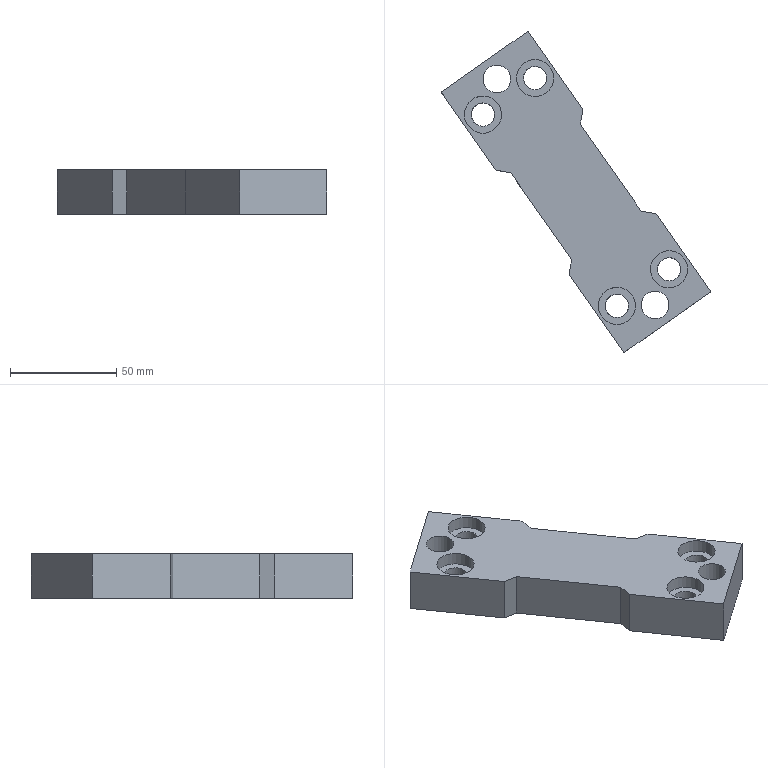Part | NX | features solid 2 | 1 solid | 28 faces | box 126.994 x 151.552 x 21 mm | volume 128901 mm3 | plane 18 | cylinder 10 | commonest cylinder face diameters 11 x4 17.5 x4 13 x2
STEP:
#1=CARTESIAN_POINT('',(-717.56,109.472,-44.));
#2=VERTEX_POINT('',#1);
#3=CARTESIAN_POINT('',(-722.579,116.64,-44.));
#4=DIRECTION('',(0.,0.,-1.));
#5=DIRECTION('',(0.5736,-0.8192,0.));
#6=AXIS2_PLACEMENT_3D('',#3,#4,#5);
#7=CIRCLE('',#6,8.75);
#8=EDGE_CURVE('',#2,#2,#7,.T.);
#9=ORIENTED_EDGE('',*,*,#8,.T.);
#10=EDGE_LOOP('',(#9));
#11=FACE_BOUND('',#10,.T.);
#12=CARTESIAN_POINT('',(-654.467,19.366,-44.));
#13=VERTEX_POINT('',#12);
#14=CARTESIAN_POINT('',(-659.485,26.533,-44.));
#15=DIRECTION('',(0.,0.,-1.));
#16=DIRECTION('',(0.5736,-0.8192,0.));
#17=AXIS2_PLACEMENT_3D('',#14,#15,#16);
#18=CIRCLE('',#17,8.75);
#19=EDGE_CURVE('',#13,#13,#18,.T.);
#20=ORIENTED_EDGE('',*,*,#19,.T.);
#21=EDGE_LOOP('',(#20));
#22=FACE_BOUND('',#21,.T.);
#23=CARTESIAN_POINT('',(-712.299,128.111,-44.));
#24=VERTEX_POINT('',#23);
#25=CARTESIAN_POINT('',(-716.027,133.435,-44.));
#26=DIRECTION('',(0.,0.,-1.));
#27=DIRECTION('',(0.5736,-0.8192,0.));
#28=AXIS2_PLACEMENT_3D('',#25,#26,#27);
#29=CIRCLE('',#28,6.5);
#30=EDGE_CURVE('',#24,#24,#29,.T.);
#31=ORIENTED_EDGE('',*,*,#30,.T.);
#32=EDGE_LOOP('',(#31));
#33=FACE_BOUND('',#32,.T.);
#34=CARTESIAN_POINT('',(-701.284,155.966,-44.));
#35=VERTEX_POINT('',#34);
#36=CARTESIAN_POINT('',(-742.242,127.287,-44.));
#37=VERTEX_POINT('',#36);
#38=CARTESIAN_POINT('',(-701.284,155.966,-44.));
#39=DIRECTION('',(-0.8192,-0.5736,0.));
#40=VECTOR('',#39,1000.);
#41=LINE('',#38,#40);
#42=EDGE_CURVE('',#35,#37,#41,.T.);
#43=ORIENTED_EDGE('',*,*,#42,.T.);
#44=CARTESIAN_POINT('',(-716.431,90.425,-44.));
#45=VERTEX_POINT('',#44);
#46=CARTESIAN_POINT('',(-742.242,127.287,-44.));
#47=DIRECTION('',(0.5736,-0.8192,0.));
#48=VECTOR('',#47,1000.);
#49=LINE('',#46,#48);
#50=EDGE_CURVE('',#37,#45,#49,.T.);
#51=ORIENTED_EDGE('',*,*,#50,.T.);
#52=CARTESIAN_POINT('',(-709.467,89.197,-44.));
#53=VERTEX_POINT('',#52);
#54=CARTESIAN_POINT('',(-716.431,90.425,-44.));
#55=DIRECTION('',(0.9848,-0.1736,0.));
#56=VECTOR('',#55,1000.);
#57=LINE('',#54,#56);
#58=EDGE_CURVE('',#45,#53,#57,.T.);
#59=ORIENTED_EDGE('',*,*,#58,.T.);
#60=CARTESIAN_POINT('',(-680.788,48.24,-44.));
#61=VERTEX_POINT('',#60);
#62=CARTESIAN_POINT('',(-709.467,89.197,-44.));
#63=DIRECTION('',(0.5736,-0.8192,0.));
#64=VECTOR('',#63,1000.);
#65=LINE('',#62,#64);
#66=EDGE_CURVE('',#53,#61,#65,.T.);
#67=ORIENTED_EDGE('',*,*,#66,.T.);
#68=CARTESIAN_POINT('',(-682.016,41.276,-44.));
#69=VERTEX_POINT('',#68);
#70=CARTESIAN_POINT('',(-680.788,48.24,-44.));
#71=DIRECTION('',(-0.1736,-0.9848,0.));
#72=VECTOR('',#71,1000.);
#73=LINE('',#70,#72);
#74=EDGE_CURVE('',#61,#69,#73,.T.);
#75=ORIENTED_EDGE('',*,*,#74,.T.);
#76=CARTESIAN_POINT('',(-656.205,4.414,-44.));
#77=VERTEX_POINT('',#76);
#78=CARTESIAN_POINT('',(-682.016,41.276,-44.));
#79=DIRECTION('',(0.5736,-0.8192,0.));
#80=VECTOR('',#79,1000.);
#81=LINE('',#78,#80);
#82=EDGE_CURVE('',#69,#77,#81,.T.);
#83=ORIENTED_EDGE('',*,*,#82,.T.);
#84=CARTESIAN_POINT('',(-615.248,33.093,-44.));
#85=VERTEX_POINT('',#84);
#86=CARTESIAN_POINT('',(-656.205,4.414,-44.));
#87=DIRECTION('',(0.8192,0.5736,0.));
#88=VECTOR('',#87,1000.);
#89=LINE('',#86,#88);
#90=EDGE_CURVE('',#77,#85,#89,.T.);
#91=ORIENTED_EDGE('',*,*,#90,.T.);
#92=CARTESIAN_POINT('',(-641.059,69.955,-44.));
#93=VERTEX_POINT('',#92);
#94=CARTESIAN_POINT('',(-641.059,69.955,-44.));
#95=DIRECTION('',(0.5736,-0.8192,0.));
#96=VECTOR('',#95,1000.);
#97=LINE('',#94,#96);
#98=EDGE_CURVE('',#93,#85,#97,.T.);
#99=ORIENTED_EDGE('',*,*,#98,.F.);
#100=CARTESIAN_POINT('',(-648.022,71.183,-44.));
#101=VERTEX_POINT('',#100);
#102=CARTESIAN_POINT('',(-648.022,71.183,-44.));
#103=DIRECTION('',(0.9848,-0.1736,0.));
#104=VECTOR('',#103,1000.);
#105=LINE('',#102,#104);
#106=EDGE_CURVE('',#101,#93,#105,.T.);
#107=ORIENTED_EDGE('',*,*,#106,.F.);
#108=CARTESIAN_POINT('',(-676.701,112.141,-44.));
#109=VERTEX_POINT('',#108);
#110=CARTESIAN_POINT('',(-676.701,112.141,-44.));
#111=DIRECTION('',(0.5736,-0.8192,0.));
#112=VECTOR('',#111,1000.);
#113=LINE('',#110,#112);
#114=EDGE_CURVE('',#109,#101,#113,.T.);
#115=ORIENTED_EDGE('',*,*,#114,.F.);
#116=CARTESIAN_POINT('',(-675.473,119.104,-44.));
#117=VERTEX_POINT('',#116);
#118=CARTESIAN_POINT('',(-676.701,112.141,-44.));
#119=DIRECTION('',(0.1736,0.9848,0.));
#120=VECTOR('',#119,1000.);
#121=LINE('',#118,#120);
#122=EDGE_CURVE('',#109,#117,#121,.T.);
#123=ORIENTED_EDGE('',*,*,#122,.T.);
#124=CARTESIAN_POINT('',(-701.284,155.966,-44.));
#125=DIRECTION('',(0.5736,-0.8192,0.));
#126=VECTOR('',#125,1000.);
#127=LINE('',#124,#126);
#128=EDGE_CURVE('',#35,#117,#127,.T.);
#129=ORIENTED_EDGE('',*,*,#128,.F.);
#130=EDGE_LOOP('',(#43,#51,#59,#67,#75,#83,#91,#99,#107,#115,#123,#129));
#131=FACE_BOUND('',#130,.T.);
#132=CARTESIAN_POINT('',(-637.734,21.621,-44.));
#133=VERTEX_POINT('',#132);
#134=CARTESIAN_POINT('',(-641.462,26.945,-44.));
#135=DIRECTION('',(0.,0.,-1.));
#136=DIRECTION('',(0.5736,-0.8192,0.));
#137=AXIS2_PLACEMENT_3D('',#134,#135,#136);
#138=CIRCLE('',#137,6.5);
#139=EDGE_CURVE('',#133,#133,#138,.T.);
#140=ORIENTED_EDGE('',*,*,#139,.T.);
#141=EDGE_LOOP('',(#140));
#142=FACE_BOUND('',#141,.T.);
#143=CARTESIAN_POINT('',(-629.892,36.573,-44.));
#144=VERTEX_POINT('',#143);
#145=CARTESIAN_POINT('',(-634.911,43.74,-44.));
#146=DIRECTION('',(0.,0.,-1.));
#147=DIRECTION('',(0.5736,-0.8192,0.));
#148=AXIS2_PLACEMENT_3D('',#145,#146,#147);
#149=CIRCLE('',#148,8.75);
#150=EDGE_CURVE('',#144,#144,#149,.T.);
#151=ORIENTED_EDGE('',*,*,#150,.T.);
#152=EDGE_LOOP('',(#151));
#153=FACE_BOUND('',#152,.T.);
#154=CARTESIAN_POINT('',(-692.985,126.68,-44.));
#155=VERTEX_POINT('',#154);
#156=CARTESIAN_POINT('',(-698.004,133.847,-44.));
#157=DIRECTION('',(0.,0.,-1.));
#158=DIRECTION('',(0.5736,-0.8192,0.));
#159=AXIS2_PLACEMENT_3D('',#156,#157,#158);
#160=CIRCLE('',#159,8.75);
#161=EDGE_CURVE('',#155,#155,#160,.T.);
#162=ORIENTED_EDGE('',*,*,#161,.T.);
#163=EDGE_LOOP('',(#162));
#164=FACE_BOUND('',#163,.T.);
#165=CARTESIAN_POINT('',(-742.242,127.287,-44.));
#166=DIRECTION('',(0.,0.,-1.));
#167=DIRECTION('',(-0.8192,-0.5736,0.));
#168=AXIS2_PLACEMENT_3D('',#165,#166,#167);
#169=PLANE('',#168);
#170=ADVANCED_FACE('',(#11,#22,#33,#131,#142,#153,#164),#169,.F.);
#171=CARTESIAN_POINT('',(-694.85,129.342,-65.));
#172=VERTEX_POINT('',#171);
#173=CARTESIAN_POINT('',(-698.004,133.847,-65.));
#174=DIRECTION('',(0.,0.,-1.));
#175=DIRECTION('',(0.5736,-0.8192,0.));
#176=AXIS2_PLACEMENT_3D('',#173,#174,#175);
#177=CIRCLE('',#176,5.5);
#178=EDGE_CURVE('',#172,#172,#177,.T.);
#179=ORIENTED_EDGE('',*,*,#178,.T.);
#180=EDGE_LOOP('',(#179));
#181=FACE_BOUND('',#180,.T.);
#182=CARTESIAN_POINT('',(-693.499,137.002,-50.));
#183=VERTEX_POINT('',#182);
#184=CARTESIAN_POINT('',(-698.004,133.847,-50.));
#185=DIRECTION('',(0.,0.,-1.));
#186=DIRECTION('',(0.8192,0.5736,0.));
#187=AXIS2_PLACEMENT_3D('',#184,#185,#186);
#188=CIRCLE('',#187,5.5);
#189=EDGE_CURVE('',#183,#183,#188,.T.);
#190=ORIENTED_EDGE('',*,*,#189,.F.);
#191=EDGE_LOOP('',(#190));
#192=FACE_BOUND('',#191,.T.);
#193=CARTESIAN_POINT('',(-698.004,133.847,-44.));
#194=DIRECTION('',(0.,0.,-1.));
#195=DIRECTION('',(-0.8192,-0.5736,0.));
#196=AXIS2_PLACEMENT_3D('',#193,#194,#195);
#197=CYLINDRICAL_SURFACE('',#196,5.5);
#198=ADVANCED_FACE('',(#181,#192),#197,.F.);
#199=CARTESIAN_POINT('',(-719.424,112.135,-65.));
#200=VERTEX_POINT('',#199);
#201=CARTESIAN_POINT('',(-722.579,116.64,-65.));
#202=DIRECTION('',(0.,0.,-1.));
#203=DIRECTION('',(0.5736,-0.8192,0.));
#204=AXIS2_PLACEMENT_3D('',#201,#202,#203);
#205=CIRCLE('',#204,5.5);
#206=EDGE_CURVE('',#200,#200,#205,.T.);
#207=ORIENTED_EDGE('',*,*,#206,.T.);
#208=EDGE_LOOP('',(#207));
#209=FACE_BOUND('',#208,.T.);
#210=CARTESIAN_POINT('',(-718.073,119.795,-50.));
#211=VERTEX_POINT('',#210);
#212=CARTESIAN_POINT('',(-722.579,116.64,-50.));
#213=DIRECTION('',(0.,0.,-1.));
#214=DIRECTION('',(0.8192,0.5736,0.));
#215=AXIS2_PLACEMENT_3D('',#212,#213,#214);
#216=CIRCLE('',#215,5.5);
#217=EDGE_CURVE('',#211,#211,#216,.T.);
#218=ORIENTED_EDGE('',*,*,#217,.F.);
#219=EDGE_LOOP('',(#218));
#220=FACE_BOUND('',#219,.T.);
#221=CARTESIAN_POINT('',(-722.579,116.64,-44.));
#222=DIRECTION('',(0.,0.,-1.));
#223=DIRECTION('',(-0.8192,-0.5736,0.));
#224=AXIS2_PLACEMENT_3D('',#221,#222,#223);
#225=CYLINDRICAL_SURFACE('',#224,5.5);
#226=ADVANCED_FACE('',(#209,#220),#225,.F.);
#227=CARTESIAN_POINT('',(-631.756,39.235,-65.));
#228=VERTEX_POINT('',#227);
#229=CARTESIAN_POINT('',(-634.911,43.74,-65.));
#230=DIRECTION('',(0.,0.,-1.));
#231=DIRECTION('',(0.5736,-0.8192,0.));
#232=AXIS2_PLACEMENT_3D('',#229,#230,#231);
#233=CIRCLE('',#232,5.5);
#234=EDGE_CURVE('',#228,#228,#233,.T.);
#235=ORIENTED_EDGE('',*,*,#234,.T.);
#236=EDGE_LOOP('',(#235));
#237=FACE_BOUND('',#236,.T.);
#238=CARTESIAN_POINT('',(-630.406,46.895,-50.));
#239=VERTEX_POINT('',#238);
#240=CARTESIAN_POINT('',(-634.911,43.74,-50.));
#241=DIRECTION('',(0.,0.,-1.));
#242=DIRECTION('',(0.8192,0.5736,0.));
#243=AXIS2_PLACEMENT_3D('',#240,#241,#242);
#244=CIRCLE('',#243,5.5);
#245=EDGE_CURVE('',#239,#239,#244,.T.);
#246=ORIENTED_EDGE('',*,*,#245,.F.);
#247=EDGE_LOOP('',(#246));
#248=FACE_BOUND('',#247,.T.);
#249=CARTESIAN_POINT('',(-634.911,43.74,-44.));
#250=DIRECTION('',(0.,0.,-1.));
#251=DIRECTION('',(-0.8192,-0.5736,0.));
#252=AXIS2_PLACEMENT_3D('',#249,#250,#251);
#253=CYLINDRICAL_SURFACE('',#252,5.5);
#254=ADVANCED_FACE('',(#237,#248),#253,.F.);
#255=CARTESIAN_POINT('',(-656.331,22.028,-65.));
#256=VERTEX_POINT('',#255);
#257=CARTESIAN_POINT('',(-659.485,26.533,-65.));
#258=DIRECTION('',(0.,0.,-1.));
#259=DIRECTION('',(0.5736,-0.8192,0.));
#260=AXIS2_PLACEMENT_3D('',#257,#258,#259);
#261=CIRCLE('',#260,5.5);
#262=EDGE_CURVE('',#256,#256,#261,.T.);
#263=ORIENTED_EDGE('',*,*,#262,.T.);
#264=EDGE_LOOP('',(#263));
#265=FACE_BOUND('',#264,.T.);
#266=CARTESIAN_POINT('',(-654.98,29.688,-50.));
#267=VERTEX_POINT('',#266);
#268=CARTESIAN_POINT('',(-659.485,26.533,-50.));
#269=DIRECTION('',(0.,0.,-1.));
#270=DIRECTION('',(0.8192,0.5736,0.));
#271=AXIS2_PLACEMENT_3D('',#268,#269,#270);
#272=CIRCLE('',#271,5.5);
#273=EDGE_CURVE('',#267,#267,#272,.T.);
#274=ORIENTED_EDGE('',*,*,#273,.F.);
#275=EDGE_LOOP('',(#274));
#276=FACE_BOUND('',#275,.T.);
#277=CARTESIAN_POINT('',(-659.485,26.533,-44.));
#278=DIRECTION('',(0.,0.,-1.));
#279=DIRECTION('',(-0.8192,-0.5736,0.));
#280=AXIS2_PLACEMENT_3D('',#277,#278,#279);
#281=CYLINDRICAL_SURFACE('',#280,5.5);
#282=ADVANCED_FACE('',(#265,#276),#281,.F.);
#283=CARTESIAN_POINT('',(-712.299,128.111,-65.));
#284=VERTEX_POINT('',#283);
#285=CARTESIAN_POINT('',(-716.027,133.435,-65.));
#286=DIRECTION('',(0.,0.,-1.));
#287=DIRECTION('',(0.5736,-0.8192,0.));
#288=AXIS2_PLACEMENT_3D('',#285,#286,#287);
#289=CIRCLE('',#288,6.5);
#290=EDGE_CURVE('',#284,#284,#289,.T.);
#291=ORIENTED_EDGE('',*,*,#290,.F.);
#292=EDGE_LOOP('',(#291));
#293=FACE_BOUND('',#292,.T.);
#294=ORIENTED_EDGE('',*,*,#234,.F.);
#295=EDGE_LOOP('',(#294));
#296=FACE_BOUND('',#295,.T.);
#297=ORIENTED_EDGE('',*,*,#262,.F.);
#298=EDGE_LOOP('',(#297));
#299=FACE_BOUND('',#298,.T.);
#300=CARTESIAN_POINT('',(-701.284,155.966,-65.));
#301=VERTEX_POINT('',#300);
#302=CARTESIAN_POINT('',(-742.242,127.287,-65.));
#303=VERTEX_POINT('',#302);
#304=CARTESIAN_POINT('',(-701.284,155.966,-65.));
#305=DIRECTION('',(-0.8192,-0.5736,0.));
#306=VECTOR('',#305,1000.);
#307=LINE('',#304,#306);
#308=EDGE_CURVE('',#301,#303,#307,.T.);
#309=ORIENTED_EDGE('',*,*,#308,.F.);
#310=CARTESIAN_POINT('',(-675.473,119.104,-65.));
#311=VERTEX_POINT('',#310);
#312=CARTESIAN_POINT('',(-701.284,155.966,-65.));
#313=DIRECTION('',(0.5736,-0.8192,0.));
#314=VECTOR('',#313,1000.);
#315=LINE('',#312,#314);
#316=EDGE_CURVE('',#301,#311,#315,.T.);
#317=ORIENTED_EDGE('',*,*,#316,.T.);
#318=CARTESIAN_POINT('',(-676.701,112.141,-65.));
#319=VERTEX_POINT('',#318);
#320=CARTESIAN_POINT('',(-676.701,112.141,-65.));
#321=DIRECTION('',(0.1736,0.9848,0.));
#322=VECTOR('',#321,1000.);
#323=LINE('',#320,#322);
#324=EDGE_CURVE('',#319,#311,#323,.T.);
#325=ORIENTED_EDGE('',*,*,#324,.F.);
#326=CARTESIAN_POINT('',(-648.022,71.183,-65.));
#327=VERTEX_POINT('',#326);
#328=CARTESIAN_POINT('',(-676.701,112.141,-65.));
#329=DIRECTION('',(0.5736,-0.8192,0.));
#330=VECTOR('',#329,1000.);
#331=LINE('',#328,#330);
#332=EDGE_CURVE('',#319,#327,#331,.T.);
#333=ORIENTED_EDGE('',*,*,#332,.T.);
#334=CARTESIAN_POINT('',(-641.059,69.955,-65.));
#335=VERTEX_POINT('',#334);
#336=CARTESIAN_POINT('',(-648.022,71.183,-65.));
#337=DIRECTION('',(0.9848,-0.1736,0.));
#338=VECTOR('',#337,1000.);
#339=LINE('',#336,#338);
#340=EDGE_CURVE('',#327,#335,#339,.T.);
#341=ORIENTED_EDGE('',*,*,#340,.T.);
#342=CARTESIAN_POINT('',(-615.248,33.093,-65.));
#343=VERTEX_POINT('',#342);
#344=CARTESIAN_POINT('',(-641.059,69.955,-65.));
#345=DIRECTION('',(0.5736,-0.8192,0.));
#346=VECTOR('',#345,1000.);
#347=LINE('',#344,#346);
#348=EDGE_CURVE('',#335,#343,#347,.T.);
#349=ORIENTED_EDGE('',*,*,#348,.T.);
#350=CARTESIAN_POINT('',(-656.205,4.414,-65.));
#351=VERTEX_POINT('',#350);
#352=CARTESIAN_POINT('',(-656.205,4.414,-65.));
#353=DIRECTION('',(0.8192,0.5736,0.));
#354=VECTOR('',#353,1000.);
#355=LINE('',#352,#354);
#356=EDGE_CURVE('',#351,#343,#355,.T.);
#357=ORIENTED_EDGE('',*,*,#356,.F.);
#358=CARTESIAN_POINT('',(-682.016,41.276,-65.));
#359=VERTEX_POINT('',#358);
#360=CARTESIAN_POINT('',(-682.016,41.276,-65.));
#361=DIRECTION('',(0.5736,-0.8192,0.));
#362=VECTOR('',#361,1000.);
#363=LINE('',#360,#362);
#364=EDGE_CURVE('',#359,#351,#363,.T.);
#365=ORIENTED_EDGE('',*,*,#364,.F.);
#366=CARTESIAN_POINT('',(-680.788,48.24,-65.));
#367=VERTEX_POINT('',#366);
#368=CARTESIAN_POINT('',(-680.788,48.24,-65.));
#369=DIRECTION('',(-0.1736,-0.9848,0.));
#370=VECTOR('',#369,1000.);
#371=LINE('',#368,#370);
#372=EDGE_CURVE('',#367,#359,#371,.T.);
#373=ORIENTED_EDGE('',*,*,#372,.F.);
#374=CARTESIAN_POINT('',(-709.467,89.197,-65.));
#375=VERTEX_POINT('',#374);
#376=CARTESIAN_POINT('',(-709.467,89.197,-65.));
#377=DIRECTION('',(0.5736,-0.8192,0.));
#378=VECTOR('',#377,1000.);
#379=LINE('',#376,#378);
#380=EDGE_CURVE('',#375,#367,#379,.T.);
#381=ORIENTED_EDGE('',*,*,#380,.F.);
#382=CARTESIAN_POINT('',(-716.431,90.425,-65.));
#383=VERTEX_POINT('',#382);
#384=CARTESIAN_POINT('',(-716.431,90.425,-65.));
#385=DIRECTION('',(0.9848,-0.1736,0.));
#386=VECTOR('',#385,1000.);
#387=LINE('',#384,#386);
#388=EDGE_CURVE('',#383,#375,#387,.T.);
#389=ORIENTED_EDGE('',*,*,#388,.F.);
#390=CARTESIAN_POINT('',(-742.242,127.287,-65.));
#391=DIRECTION('',(0.5736,-0.8192,0.));
#392=VECTOR('',#391,1000.);
#393=LINE('',#390,#392);
#394=EDGE_CURVE('',#303,#383,#393,.T.);
#395=ORIENTED_EDGE('',*,*,#394,.F.);
#396=EDGE_LOOP('',(#309,#317,#325,#333,#341,#349,#357,#365,#373,#381,#389,#395));
#397=FACE_BOUND('',#396,.T.);
#398=CARTESIAN_POINT('',(-637.734,21.621,-65.));
#399=VERTEX_POINT('',#398);
#400=CARTESIAN_POINT('',(-641.462,26.945,-65.));
#401=DIRECTION('',(0.,0.,-1.));
#402=DIRECTION('',(0.5736,-0.8192,0.));
#403=AXIS2_PLACEMENT_3D('',#400,#401,#402);
#404=CIRCLE('',#403,6.5);
#405=EDGE_CURVE('',#399,#399,#404,.T.);
#406=ORIENTED_EDGE('',*,*,#405,.F.);
#407=EDGE_LOOP('',(#406));
#408=FACE_BOUND('',#407,.T.);
#409=ORIENTED_EDGE('',*,*,#206,.F.);
#410=EDGE_LOOP('',(#409));
#411=FACE_BOUND('',#410,.T.);
#412=ORIENTED_EDGE('',*,*,#178,.F.);
#413=EDGE_LOOP('',(#412));
#414=FACE_BOUND('',#413,.T.);
#415=CARTESIAN_POINT('',(-742.242,127.287,-65.));
#416=DIRECTION('',(0.,0.,-1.));
#417=DIRECTION('',(-0.8192,-0.5736,0.));
#418=AXIS2_PLACEMENT_3D('',#415,#416,#417);
#419=PLANE('',#418);
#420=ADVANCED_FACE('',(#293,#296,#299,#397,#408,#411,#414),#419,.T.);
#421=ORIENTED_EDGE('',*,*,#308,.T.);
#422=CARTESIAN_POINT('',(-742.242,127.287,-44.));
#423=DIRECTION('',(0.,0.,-1.));
#424=VECTOR('',#423,1000.);
#425=LINE('',#422,#424);
#426=EDGE_CURVE('',#37,#303,#425,.T.);
#427=ORIENTED_EDGE('',*,*,#426,.F.);
#428=ORIENTED_EDGE('',*,*,#42,.F.);
#429=CARTESIAN_POINT('',(-701.284,155.966,-44.));
#430=DIRECTION('',(0.,0.,-1.));
#431=VECTOR('',#430,1000.);
#432=LINE('',#429,#431);
#433=EDGE_CURVE('',#35,#301,#432,.T.);
#434=ORIENTED_EDGE('',*,*,#433,.T.);
#435=EDGE_LOOP('',(#421,#427,#428,#434));
#436=FACE_BOUND('',#435,.T.);
#437=CARTESIAN_POINT('',(-701.284,155.966,-44.));
#438=DIRECTION('',(-0.5736,0.8192,0.));
#439=DIRECTION('',(0.8192,0.5736,0.));
#440=AXIS2_PLACEMENT_3D('',#437,#438,#439);
#441=PLANE('',#440);
#442=ADVANCED_FACE('',(#436),#441,.T.);
#443=ORIENTED_EDGE('',*,*,#394,.T.);
#444=CARTESIAN_POINT('',(-716.431,90.425,-44.));
#445=DIRECTION('',(0.,0.,-1.));
#446=VECTOR('',#445,1000.);
#447=LINE('',#444,#446);
#448=EDGE_CURVE('',#45,#383,#447,.T.);
#449=ORIENTED_EDGE('',*,*,#448,.F.);
#450=ORIENTED_EDGE('',*,*,#50,.F.);
#451=ORIENTED_EDGE('',*,*,#426,.T.);
#452=EDGE_LOOP('',(#443,#449,#450,#451));
#453=FACE_BOUND('',#452,.T.);
#454=CARTESIAN_POINT('',(-742.242,127.287,-44.));
#455=DIRECTION('',(-0.8192,-0.5736,0.));
#456=DIRECTION('',(-0.5736,0.8192,0.));
#457=AXIS2_PLACEMENT_3D('',#454,#455,#456);
#458=PLANE('',#457);
#459=ADVANCED_FACE('',(#453),#458,.T.);
#460=ORIENTED_EDGE('',*,*,#388,.T.);
#461=CARTESIAN_POINT('',(-709.467,89.197,-44.));
#462=DIRECTION('',(0.,0.,-1.));
#463=VECTOR('',#462,1000.);
#464=LINE('',#461,#463);
#465=EDGE_CURVE('',#53,#375,#464,.T.);
#466=ORIENTED_EDGE('',*,*,#465,.F.);
#467=ORIENTED_EDGE('',*,*,#58,.F.);
#468=ORIENTED_EDGE('',*,*,#448,.T.);
#469=EDGE_LOOP('',(#460,#466,#467,#468));
#470=FACE_BOUND('',#469,.T.);
#471=CARTESIAN_POINT('',(-716.431,90.425,-44.));
#472=DIRECTION('',(-0.1736,-0.9848,0.));
#473=DIRECTION('',(-0.9848,0.1736,0.));
#474=AXIS2_PLACEMENT_3D('',#471,#472,#473);
#475=PLANE('',#474);
#476=ADVANCED_FACE('',(#470),#475,.T.);
#477=ORIENTED_EDGE('',*,*,#380,.T.);
#478=CARTESIAN_POINT('',(-680.788,48.24,-44.));
#479=DIRECTION('',(0.,0.,-1.));
#480=VECTOR('',#479,1000.);
#481=LINE('',#478,#480);
#482=EDGE_CURVE('',#61,#367,#481,.T.);
#483=ORIENTED_EDGE('',*,*,#482,.F.);
#484=ORIENTED_EDGE('',*,*,#66,.F.);
#485=ORIENTED_EDGE('',*,*,#465,.T.);
#486=EDGE_LOOP('',(#477,#483,#484,#485));
#487=FACE_BOUND('',#486,.T.);
#488=CARTESIAN_POINT('',(-709.467,89.197,-44.));
#489=DIRECTION('',(-0.8192,-0.5736,0.));
#490=DIRECTION('',(-0.5736,0.8192,0.));
#491=AXIS2_PLACEMENT_3D('',#488,#489,#490);
#492=PLANE('',#491);
#493=ADVANCED_FACE('',(#487),#492,.T.);
#494=ORIENTED_EDGE('',*,*,#372,.T.);
#495=CARTESIAN_POINT('',(-682.016,41.276,-44.));
#496=DIRECTION('',(0.,0.,-1.));
#497=VECTOR('',#496,1000.);
#498=LINE('',#495,#497);
#499=EDGE_CURVE('',#69,#359,#498,.T.);
#500=ORIENTED_EDGE('',*,*,#499,.F.);
#501=ORIENTED_EDGE('',*,*,#74,.F.);
#502=ORIENTED_EDGE('',*,*,#482,.T.);
#503=EDGE_LOOP('',(#494,#500,#501,#502));
#504=FACE_BOUND('',#503,.T.);
#505=CARTESIAN_POINT('',(-680.788,48.24,-44.));
#506=DIRECTION('',(-0.9848,0.1736,0.));
#507=DIRECTION('',(0.1736,0.9848,0.));
#508=AXIS2_PLACEMENT_3D('',#505,#506,#507);
#509=PLANE('',#508);
#510=ADVANCED_FACE('',(#504),#509,.T.);
#511=ORIENTED_EDGE('',*,*,#364,.T.);
#512=CARTESIAN_POINT('',(-656.205,4.414,-44.));
#513=DIRECTION('',(0.,0.,-1.));
#514=VECTOR('',#513,1000.);
#515=LINE('',#512,#514);
#516=EDGE_CURVE('',#77,#351,#515,.T.);
#517=ORIENTED_EDGE('',*,*,#516,.F.);
#518=ORIENTED_EDGE('',*,*,#82,.F.);
#519=ORIENTED_EDGE('',*,*,#499,.T.);
#520=EDGE_LOOP('',(#511,#517,#518,#519));
#521=FACE_BOUND('',#520,.T.);
#522=CARTESIAN_POINT('',(-682.016,41.276,-44.));
#523=DIRECTION('',(-0.8192,-0.5736,0.));
#524=DIRECTION('',(-0.5736,0.8192,0.));
#525=AXIS2_PLACEMENT_3D('',#522,#523,#524);
#526=PLANE('',#525);
#527=ADVANCED_FACE('',(#521),#526,.T.);
#528=ORIENTED_EDGE('',*,*,#356,.T.);
#529=CARTESIAN_POINT('',(-615.248,33.093,-44.));
#530=DIRECTION('',(0.,0.,-1.));
#531=VECTOR('',#530,1000.);
#532=LINE('',#529,#531);
#533=EDGE_CURVE('',#85,#343,#532,.T.);
#534=ORIENTED_EDGE('',*,*,#533,.F.);
#535=ORIENTED_EDGE('',*,*,#90,.F.);
#536=ORIENTED_EDGE('',*,*,#516,.T.);
#537=EDGE_LOOP('',(#528,#534,#535,#536));
#538=FACE_BOUND('',#537,.T.);
#539=CARTESIAN_POINT('',(-656.205,4.414,-44.));
#540=DIRECTION('',(0.5736,-0.8192,0.));
#541=DIRECTION('',(-0.8192,-0.5736,0.));
#542=AXIS2_PLACEMENT_3D('',#539,#540,#541);
#543=PLANE('',#542);
#544=ADVANCED_FACE('',(#538),#543,.T.);
#545=ORIENTED_EDGE('',*,*,#348,.F.);
#546=CARTESIAN_POINT('',(-641.059,69.955,-44.));
#547=DIRECTION('',(0.,0.,-1.));
#548=VECTOR('',#547,1000.);
#549=LINE('',#546,#548);
#550=EDGE_CURVE('',#93,#335,#549,.T.);
#551=ORIENTED_EDGE('',*,*,#550,.F.);
#552=ORIENTED_EDGE('',*,*,#98,.T.);
#553=ORIENTED_EDGE('',*,*,#533,.T.);
#554=EDGE_LOOP('',(#545,#551,#552,#553));
#555=FACE_BOUND('',#554,.T.);
#556=CARTESIAN_POINT('',(-641.059,69.955,-44.));
#557=DIRECTION('',(-0.8192,-0.5736,0.));
#558=DIRECTION('',(-0.5736,0.8192,0.));
#559=AXIS2_PLACEMENT_3D('',#556,#557,#558);
#560=PLANE('',#559);
#561=ADVANCED_FACE('',(#555),#560,.F.);
#562=ORIENTED_EDGE('',*,*,#340,.F.);
#563=CARTESIAN_POINT('',(-648.022,71.183,-44.));
#564=DIRECTION('',(0.,0.,-1.));
#565=VECTOR('',#564,1000.);
#566=LINE('',#563,#565);
#567=EDGE_CURVE('',#101,#327,#566,.T.);
#568=ORIENTED_EDGE('',*,*,#567,.F.);
#569=ORIENTED_EDGE('',*,*,#106,.T.);
#570=ORIENTED_EDGE('',*,*,#550,.T.);
#571=EDGE_LOOP('',(#562,#568,#569,#570));
#572=FACE_BOUND('',#571,.T.);
#573=CARTESIAN_POINT('',(-648.022,71.183,-44.));
#574=DIRECTION('',(-0.1736,-0.9848,0.));
#575=DIRECTION('',(-0.9848,0.1736,0.));
#576=AXIS2_PLACEMENT_3D('',#573,#574,#575);
#577=PLANE('',#576);
#578=ADVANCED_FACE('',(#572),#577,.F.);
#579=ORIENTED_EDGE('',*,*,#332,.F.);
#580=CARTESIAN_POINT('',(-676.701,112.141,-44.));
#581=DIRECTION('',(0.,0.,-1.));
#582=VECTOR('',#581,1000.);
#583=LINE('',#580,#582);
#584=EDGE_CURVE('',#109,#319,#583,.T.);
#585=ORIENTED_EDGE('',*,*,#584,.F.);
#586=ORIENTED_EDGE('',*,*,#114,.T.);
#587=ORIENTED_EDGE('',*,*,#567,.T.);
#588=EDGE_LOOP('',(#579,#585,#586,#587));
#589=FACE_BOUND('',#588,.T.);
#590=CARTESIAN_POINT('',(-676.701,112.141,-44.));
#591=DIRECTION('',(-0.8192,-0.5736,0.));
#592=DIRECTION('',(-0.5736,0.8192,0.));
#593=AXIS2_PLACEMENT_3D('',#590,#591,#592);
#594=PLANE('',#593);
#595=ADVANCED_FACE('',(#589),#594,.F.);
#596=ORIENTED_EDGE('',*,*,#324,.T.);
#597=CARTESIAN_POINT('',(-675.473,119.104,-44.));
#598=DIRECTION('',(0.,0.,-1.));
#599=VECTOR('',#598,1000.);
#600=LINE('',#597,#599);
#601=EDGE_CURVE('',#117,#311,#600,.T.);
#602=ORIENTED_EDGE('',*,*,#601,.F.);
#603=ORIENTED_EDGE('',*,*,#122,.F.);
#604=ORIENTED_EDGE('',*,*,#584,.T.);
#605=EDGE_LOOP('',(#596,#602,#603,#604));
#606=FACE_BOUND('',#605,.T.);
#607=CARTESIAN_POINT('',(-676.701,112.141,-44.));
#608=DIRECTION('',(0.9848,-0.1736,0.));
#609=DIRECTION('',(-0.1736,-0.9848,0.));
#610=AXIS2_PLACEMENT_3D('',#607,#608,#609);
#611=PLANE('',#610);
#612=ADVANCED_FACE('',(#606),#611,.T.);
#613=ORIENTED_EDGE('',*,*,#316,.F.);
#614=ORIENTED_EDGE('',*,*,#433,.F.);
#615=ORIENTED_EDGE('',*,*,#128,.T.);
#616=ORIENTED_EDGE('',*,*,#601,.T.);
#617=EDGE_LOOP('',(#613,#614,#615,#616));
#618=FACE_BOUND('',#617,.T.);
#619=CARTESIAN_POINT('',(-701.284,155.966,-44.));
#620=DIRECTION('',(-0.8192,-0.5736,0.));
#621=DIRECTION('',(-0.5736,0.8192,0.));
#622=AXIS2_PLACEMENT_3D('',#619,#620,#621);
#623=PLANE('',#622);
#624=ADVANCED_FACE('',(#618),#623,.F.);
#625=ORIENTED_EDGE('',*,*,#139,.F.);
#626=EDGE_LOOP('',(#625));
#627=FACE_BOUND('',#626,.T.);
#628=ORIENTED_EDGE('',*,*,#405,.T.);
#629=EDGE_LOOP('',(#628));
#630=FACE_BOUND('',#629,.T.);
#631=CARTESIAN_POINT('',(-641.462,26.945,-44.));
#632=DIRECTION('',(0.,0.,-1.));
#633=DIRECTION('',(-0.8192,-0.5736,0.));
#634=AXIS2_PLACEMENT_3D('',#631,#632,#633);
#635=CYLINDRICAL_SURFACE('',#634,6.5);
#636=ADVANCED_FACE('',(#627,#630),#635,.F.);
#637=ORIENTED_EDGE('',*,*,#30,.F.);
#638=EDGE_LOOP('',(#637));
#639=FACE_BOUND('',#638,.T.);
#640=ORIENTED_EDGE('',*,*,#290,.T.);
#641=EDGE_LOOP('',(#640));
#642=FACE_BOUND('',#641,.T.);
#643=CARTESIAN_POINT('',(-716.027,133.435,-44.));
#644=DIRECTION('',(0.,0.,-1.));
#645=DIRECTION('',(-0.8192,-0.5736,0.));
#646=AXIS2_PLACEMENT_3D('',#643,#644,#645);
#647=CYLINDRICAL_SURFACE('',#646,6.5);
#648=ADVANCED_FACE('',(#639,#642),#647,.F.);
#649=ORIENTED_EDGE('',*,*,#19,.F.);
#650=EDGE_LOOP('',(#649));
#651=FACE_BOUND('',#650,.T.);
#652=CARTESIAN_POINT('',(-654.467,19.366,-50.));
#653=VERTEX_POINT('',#652);
#654=CARTESIAN_POINT('',(-659.485,26.533,-50.));
#655=DIRECTION('',(0.,0.,-1.));
#656=DIRECTION('',(0.5736,-0.8192,0.));
#657=AXIS2_PLACEMENT_3D('',#654,#655,#656);
#658=CIRCLE('',#657,8.75);
#659=EDGE_CURVE('',#653,#653,#658,.T.);
#660=ORIENTED_EDGE('',*,*,#659,.T.);
#661=EDGE_LOOP('',(#660));
#662=FACE_BOUND('',#661,.T.);
#663=CARTESIAN_POINT('',(-659.485,26.533,-44.));
#664=DIRECTION('',(0.,0.,-1.));
#665=DIRECTION('',(-0.8192,-0.5736,0.));
#666=AXIS2_PLACEMENT_3D('',#663,#664,#665);
#667=CYLINDRICAL_SURFACE('',#666,8.75);
#668=ADVANCED_FACE('',(#651,#662),#667,.F.);
#669=ORIENTED_EDGE('',*,*,#273,.T.);
#670=EDGE_LOOP('',(#669));
#671=FACE_BOUND('',#670,.T.);
#672=ORIENTED_EDGE('',*,*,#659,.F.);
#673=EDGE_LOOP('',(#672));
#674=FACE_BOUND('',#673,.T.);
#675=CARTESIAN_POINT('',(-659.485,26.533,-50.));
#676=DIRECTION('',(0.,0.,1.));
#677=DIRECTION('',(0.8192,0.5736,0.));
#678=AXIS2_PLACEMENT_3D('',#675,#676,#677);
#679=PLANE('',#678);
#680=ADVANCED_FACE('',(#671,#674),#679,.T.);
#681=ORIENTED_EDGE('',*,*,#150,.F.);
#682=EDGE_LOOP('',(#681));
#683=FACE_BOUND('',#682,.T.);
#684=CARTESIAN_POINT('',(-629.892,36.573,-50.));
#685=VERTEX_POINT('',#684);
#686=CARTESIAN_POINT('',(-634.911,43.74,-50.));
#687=DIRECTION('',(0.,0.,-1.));
#688=DIRECTION('',(0.5736,-0.8192,0.));
#689=AXIS2_PLACEMENT_3D('',#686,#687,#688);
#690=CIRCLE('',#689,8.75);
#691=EDGE_CURVE('',#685,#685,#690,.T.);
#692=ORIENTED_EDGE('',*,*,#691,.T.);
#693=EDGE_LOOP('',(#692));
#694=FACE_BOUND('',#693,.T.);
#695=CARTESIAN_POINT('',(-634.911,43.74,-44.));
#696=DIRECTION('',(0.,0.,-1.));
#697=DIRECTION('',(-0.8192,-0.5736,0.));
#698=AXIS2_PLACEMENT_3D('',#695,#696,#697);
#699=CYLINDRICAL_SURFACE('',#698,8.75);
#700=ADVANCED_FACE('',(#683,#694),#699,.F.);
#701=ORIENTED_EDGE('',*,*,#245,.T.);
#702=EDGE_LOOP('',(#701));
#703=FACE_BOUND('',#702,.T.);
#704=ORIENTED_EDGE('',*,*,#691,.F.);
#705=EDGE_LOOP('',(#704));
#706=FACE_BOUND('',#705,.T.);
#707=CARTESIAN_POINT('',(-634.911,43.74,-50.));
#708=DIRECTION('',(0.,0.,1.));
#709=DIRECTION('',(0.8192,0.5736,0.));
#710=AXIS2_PLACEMENT_3D('',#707,#708,#709);
#711=PLANE('',#710);
#712=ADVANCED_FACE('',(#703,#706),#711,.T.);
#713=ORIENTED_EDGE('',*,*,#8,.F.);
#714=EDGE_LOOP('',(#713));
#715=FACE_BOUND('',#714,.T.);
#716=CARTESIAN_POINT('',(-717.56,109.472,-50.));
#717=VERTEX_POINT('',#716);
#718=CARTESIAN_POINT('',(-722.579,116.64,-50.));
#719=DIRECTION('',(0.,0.,-1.));
#720=DIRECTION('',(0.5736,-0.8192,0.));
#721=AXIS2_PLACEMENT_3D('',#718,#719,#720);
#722=CIRCLE('',#721,8.75);
#723=EDGE_CURVE('',#717,#717,#722,.T.);
#724=ORIENTED_EDGE('',*,*,#723,.T.);
#725=EDGE_LOOP('',(#724));
#726=FACE_BOUND('',#725,.T.);
#727=CARTESIAN_POINT('',(-722.579,116.64,-44.));
#728=DIRECTION('',(0.,0.,-1.));
#729=DIRECTION('',(-0.8192,-0.5736,0.));
#730=AXIS2_PLACEMENT_3D('',#727,#728,#729);
#731=CYLINDRICAL_SURFACE('',#730,8.75);
#732=ADVANCED_FACE('',(#715,#726),#731,.F.);
#733=ORIENTED_EDGE('',*,*,#217,.T.);
#734=EDGE_LOOP('',(#733));
#735=FACE_BOUND('',#734,.T.);
#736=ORIENTED_EDGE('',*,*,#723,.F.);
#737=EDGE_LOOP('',(#736));
#738=FACE_BOUND('',#737,.T.);
#739=CARTESIAN_POINT('',(-722.579,116.64,-50.));
#740=DIRECTION('',(0.,0.,1.));
#741=DIRECTION('',(0.8192,0.5736,0.));
#742=AXIS2_PLACEMENT_3D('',#739,#740,#741);
#743=PLANE('',#742);
#744=ADVANCED_FACE('',(#735,#738),#743,.T.);
#745=ORIENTED_EDGE('',*,*,#161,.F.);
#746=EDGE_LOOP('',(#745));
#747=FACE_BOUND('',#746,.T.);
#748=CARTESIAN_POINT('',(-692.985,126.68,-50.));
#749=VERTEX_POINT('',#748);
#750=CARTESIAN_POINT('',(-698.004,133.847,-50.));
#751=DIRECTION('',(0.,0.,-1.));
#752=DIRECTION('',(0.5736,-0.8192,0.));
#753=AXIS2_PLACEMENT_3D('',#750,#751,#752);
#754=CIRCLE('',#753,8.75);
#755=EDGE_CURVE('',#749,#749,#754,.T.);
#756=ORIENTED_EDGE('',*,*,#755,.T.);
#757=EDGE_LOOP('',(#756));
#758=FACE_BOUND('',#757,.T.);
#759=CARTESIAN_POINT('',(-698.004,133.847,-44.));
#760=DIRECTION('',(0.,0.,-1.));
#761=DIRECTION('',(-0.8192,-0.5736,0.));
#762=AXIS2_PLACEMENT_3D('',#759,#760,#761);
#763=CYLINDRICAL_SURFACE('',#762,8.75);
#764=ADVANCED_FACE('',(#747,#758),#763,.F.);
#765=ORIENTED_EDGE('',*,*,#189,.T.);
#766=EDGE_LOOP('',(#765));
#767=FACE_BOUND('',#766,.T.);
#768=ORIENTED_EDGE('',*,*,#755,.F.);
#769=EDGE_LOOP('',(#768));
#770=FACE_BOUND('',#769,.T.);
#771=CARTESIAN_POINT('',(-698.004,133.847,-50.));
#772=DIRECTION('',(0.,0.,1.));
#773=DIRECTION('',(0.8192,0.5736,0.));
#774=AXIS2_PLACEMENT_3D('',#771,#772,#773);
#775=PLANE('',#774);
#776=ADVANCED_FACE('',(#767,#770),#775,.T.);
#777=CLOSED_SHELL('',(#170,#198,#226,#254,#282,#420,#442,#459,#476,#493,#510,#527,#544,#561,#578,#595,#612,#624,#636,#648,#668,#680,#700,#712,#732,#744,#764,#776));
#778=MANIFOLD_SOLID_BREP('',#777);
#779=(LENGTH_UNIT()NAMED_UNIT(*)SI_UNIT(.MILLI.,.METRE.));
#780=UNCERTAINTY_MEASURE_WITH_UNIT(LENGTH_MEASURE(0.00001),#779,'','');
#781=(NAMED_UNIT(*)PLANE_ANGLE_UNIT()SI_UNIT($,.RADIAN.));
#782=(NAMED_UNIT(*)SI_UNIT($,.STERADIAN.)SOLID_ANGLE_UNIT());
#783=(GEOMETRIC_REPRESENTATION_CONTEXT(3)GLOBAL_UNCERTAINTY_ASSIGNED_CONTEXT((#780))GLOBAL_UNIT_ASSIGNED_CONTEXT((#779,#781,#782))REPRESENTATION_CONTEXT('',''));
#784=ADVANCED_BREP_SHAPE_REPRESENTATION('',(#778),#783);